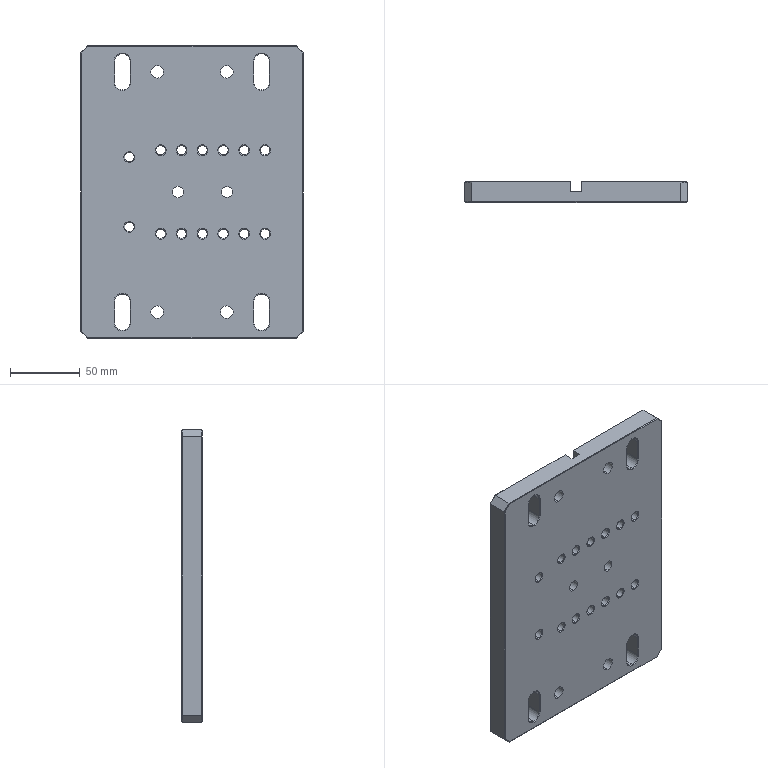Part | SolidWorks | features HoleWzd 4, Chamfer 2, Cut 2, ICE 2, LPattern 2, Extrusion 1, LibraryFeature 1 | 1 solid | 190 faces | box 160 x 15 x 210 mm | volume 461723 mm3 | cone 80 | plane 58 | cylinder 52 | commonest cylinder face diameters 6.8 x28 11 x12 9 x8 8 x4